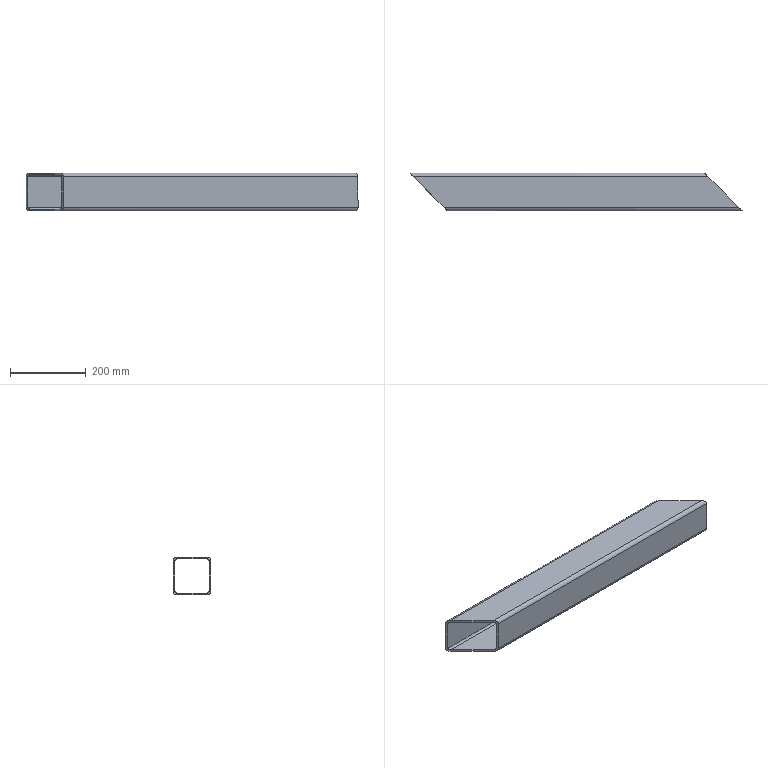Part | SolidWorks | features 3DProfileFeature 1, ICE 1, WeldMemberFeat 1, WeldmentFeature 1 | 1 solid | 18 faces | box 877.817 x 100 x 100 mm | volume 1427777 mm3 | plane 10 | cylinder 8 | commonest cylinder face diameters 10 x4 20 x4
STEP:
#1=CARTESIAN_POINT('',(777.817,50.,-40.));
#2=VERTEX_POINT('',#1);
#3=CARTESIAN_POINT('',(0.,50.,-40.));
#4=VERTEX_POINT('',#3);
#5=CARTESIAN_POINT('',(900.,50.,-40.));
#6=DIRECTION('',(-1.,0.,0.));
#7=VECTOR('',#6,1000.);
#8=LINE('',#5,#7);
#9=EDGE_CURVE('',#2,#4,#8,.T.);
#10=ORIENTED_EDGE('',*,*,#9,.F.);
#11=CARTESIAN_POINT('',(787.817,40.,-50.));
#12=VERTEX_POINT('',#11);
#13=CARTESIAN_POINT('',(777.817,50.,-40.));
#14=CARTESIAN_POINT('',(777.817,50.,-45.858));
#15=CARTESIAN_POINT('',(781.96,45.858,-50.));
#16=CARTESIAN_POINT('',(787.817,40.,-50.));
#17=(BOUNDED_CURVE()B_SPLINE_CURVE(3,(#13,#14,#15,#16),.UNSPECIFIED.,.F.,.T.)B_SPLINE_CURVE_WITH_KNOTS((4,4),(0.,1.571),.UNSPECIFIED.)CURVE()GEOMETRIC_REPRESENTATION_ITEM()RATIONAL_B_SPLINE_CURVE((1.,0.8047,0.8047,1.))REPRESENTATION_ITEM(''));
#18=EDGE_CURVE('',#2,#12,#17,.T.);
#19=ORIENTED_EDGE('',*,*,#18,.T.);
#20=CARTESIAN_POINT('',(10.,40.,-50.));
#21=VERTEX_POINT('',#20);
#22=CARTESIAN_POINT('',(900.,40.,-50.));
#23=DIRECTION('',(-1.,0.,0.));
#24=VECTOR('',#23,1000.);
#25=LINE('',#22,#24);
#26=EDGE_CURVE('',#12,#21,#25,.T.);
#27=ORIENTED_EDGE('',*,*,#26,.T.);
#28=CARTESIAN_POINT('',(10.,40.,-50.));
#29=CARTESIAN_POINT('',(4.142,45.858,-50.));
#30=CARTESIAN_POINT('',(0.,50.,-45.858));
#31=CARTESIAN_POINT('',(0.,50.,-40.));
#32=(BOUNDED_CURVE()B_SPLINE_CURVE(3,(#28,#29,#30,#31),.UNSPECIFIED.,.F.,.T.)B_SPLINE_CURVE_WITH_KNOTS((4,4),(4.712,6.283),.UNSPECIFIED.)CURVE()GEOMETRIC_REPRESENTATION_ITEM()RATIONAL_B_SPLINE_CURVE((1.,0.8047,0.8047,1.))REPRESENTATION_ITEM(''));
#33=EDGE_CURVE('',#21,#4,#32,.T.);
#34=ORIENTED_EDGE('',*,*,#33,.T.);
#35=EDGE_LOOP('',(#10,#19,#27,#34));
#36=FACE_OUTER_BOUND('',#35,.T.);
#37=CARTESIAN_POINT('',(900.,40.,-40.));
#38=DIRECTION('',(-1.,0.,0.));
#39=DIRECTION('',(0.,0.,1.));
#40=AXIS2_PLACEMENT_3D('',#37,#38,#39);
#41=CYLINDRICAL_SURFACE('',#40,10.);
#42=ADVANCED_FACE('',(#36),#41,.T.);
#43=CARTESIAN_POINT('',(777.817,50.,40.));
#44=VERTEX_POINT('',#43);
#45=CARTESIAN_POINT('',(0.,50.,40.));
#46=VERTEX_POINT('',#45);
#47=CARTESIAN_POINT('',(900.,50.,40.));
#48=DIRECTION('',(-1.,0.,0.));
#49=VECTOR('',#48,1000.);
#50=LINE('',#47,#49);
#51=EDGE_CURVE('',#44,#46,#50,.T.);
#52=ORIENTED_EDGE('',*,*,#51,.F.);
#53=CARTESIAN_POINT('',(777.817,50.,-50.));
#54=DIRECTION('',(0.,0.,1.));
#55=VECTOR('',#54,1000.);
#56=LINE('',#53,#55);
#57=EDGE_CURVE('',#2,#44,#56,.T.);
#58=ORIENTED_EDGE('',*,*,#57,.F.);
#59=ORIENTED_EDGE('',*,*,#9,.T.);
#60=CARTESIAN_POINT('',(0.,50.,-40.));
#61=DIRECTION('',(0.,0.,1.));
#62=VECTOR('',#61,1000.);
#63=LINE('',#60,#62);
#64=EDGE_CURVE('',#4,#46,#63,.T.);
#65=ORIENTED_EDGE('',*,*,#64,.T.);
#66=EDGE_LOOP('',(#52,#58,#59,#65));
#67=FACE_OUTER_BOUND('',#66,.T.);
#68=CARTESIAN_POINT('',(900.,50.,-40.));
#69=DIRECTION('',(0.,-1.,0.));
#70=DIRECTION('',(0.,0.,-1.));
#71=AXIS2_PLACEMENT_3D('',#68,#69,#70);
#72=PLANE('',#71);
#73=ADVANCED_FACE('',(#67),#72,.F.);
#74=CARTESIAN_POINT('',(787.817,40.,50.));
#75=VERTEX_POINT('',#74);
#76=CARTESIAN_POINT('',(10.,40.,50.));
#77=VERTEX_POINT('',#76);
#78=CARTESIAN_POINT('',(900.,40.,50.));
#79=DIRECTION('',(-1.,0.,0.));
#80=VECTOR('',#79,1000.);
#81=LINE('',#78,#80);
#82=EDGE_CURVE('',#75,#77,#81,.T.);
#83=ORIENTED_EDGE('',*,*,#82,.F.);
#84=CARTESIAN_POINT('',(787.817,40.,50.));
#85=CARTESIAN_POINT('',(781.96,45.858,50.));
#86=CARTESIAN_POINT('',(777.817,50.,45.858));
#87=CARTESIAN_POINT('',(777.817,50.,40.));
#88=(BOUNDED_CURVE()B_SPLINE_CURVE(3,(#84,#85,#86,#87),.UNSPECIFIED.,.F.,.T.)B_SPLINE_CURVE_WITH_KNOTS((4,4),(4.712,6.283),.UNSPECIFIED.)CURVE()GEOMETRIC_REPRESENTATION_ITEM()RATIONAL_B_SPLINE_CURVE((1.,0.8047,0.8047,1.))REPRESENTATION_ITEM(''));
#89=EDGE_CURVE('',#75,#44,#88,.T.);
#90=ORIENTED_EDGE('',*,*,#89,.T.);
#91=ORIENTED_EDGE('',*,*,#51,.T.);
#92=CARTESIAN_POINT('',(0.,50.,40.));
#93=CARTESIAN_POINT('',(0.,50.,45.858));
#94=CARTESIAN_POINT('',(4.142,45.858,50.));
#95=CARTESIAN_POINT('',(10.,40.,50.));
#96=(BOUNDED_CURVE()B_SPLINE_CURVE(3,(#92,#93,#94,#95),.UNSPECIFIED.,.F.,.T.)B_SPLINE_CURVE_WITH_KNOTS((4,4),(0.,1.571),.UNSPECIFIED.)CURVE()GEOMETRIC_REPRESENTATION_ITEM()RATIONAL_B_SPLINE_CURVE((1.,0.8047,0.8047,1.))REPRESENTATION_ITEM(''));
#97=EDGE_CURVE('',#46,#77,#96,.T.);
#98=ORIENTED_EDGE('',*,*,#97,.T.);
#99=EDGE_LOOP('',(#83,#90,#91,#98));
#100=FACE_OUTER_BOUND('',#99,.T.);
#101=CARTESIAN_POINT('',(900.,40.,40.));
#102=DIRECTION('',(-1.,0.,0.));
#103=DIRECTION('',(0.,0.,1.));
#104=AXIS2_PLACEMENT_3D('',#101,#102,#103);
#105=CYLINDRICAL_SURFACE('',#104,10.);
#106=ADVANCED_FACE('',(#100),#105,.T.);
#107=CARTESIAN_POINT('',(867.817,-40.,50.));
#108=VERTEX_POINT('',#107);
#109=CARTESIAN_POINT('',(90.,-40.,50.));
#110=VERTEX_POINT('',#109);
#111=CARTESIAN_POINT('',(900.,-40.,50.));
#112=DIRECTION('',(-1.,0.,0.));
#113=VECTOR('',#112,1000.);
#114=LINE('',#111,#113);
#115=EDGE_CURVE('',#108,#110,#114,.T.);
#116=ORIENTED_EDGE('',*,*,#115,.F.);
#117=CARTESIAN_POINT('',(777.817,50.,50.));
#118=DIRECTION('',(0.7071,-0.7071,0.));
#119=VECTOR('',#118,1000.);
#120=LINE('',#117,#119);
#121=EDGE_CURVE('',#75,#108,#120,.T.);
#122=ORIENTED_EDGE('',*,*,#121,.F.);
#123=ORIENTED_EDGE('',*,*,#82,.T.);
#124=CARTESIAN_POINT('',(0.,50.,50.));
#125=DIRECTION('',(-0.7071,0.7071,0.));
#126=VECTOR('',#125,1000.);
#127=LINE('',#124,#126);
#128=EDGE_CURVE('',#110,#77,#127,.T.);
#129=ORIENTED_EDGE('',*,*,#128,.F.);
#130=EDGE_LOOP('',(#116,#122,#123,#129));
#131=FACE_OUTER_BOUND('',#130,.T.);
#132=CARTESIAN_POINT('',(900.,-40.,50.));
#133=DIRECTION('',(0.,0.,-1.));
#134=DIRECTION('',(-1.,0.,0.));
#135=AXIS2_PLACEMENT_3D('',#132,#133,#134);
#136=PLANE('',#135);
#137=ADVANCED_FACE('',(#131),#136,.F.);
#138=CARTESIAN_POINT('',(877.817,-50.,40.));
#139=VERTEX_POINT('',#138);
#140=CARTESIAN_POINT('',(100.,-50.,40.));
#141=VERTEX_POINT('',#140);
#142=CARTESIAN_POINT('',(900.,-50.,40.));
#143=DIRECTION('',(-1.,0.,0.));
#144=VECTOR('',#143,1000.);
#145=LINE('',#142,#144);
#146=EDGE_CURVE('',#139,#141,#145,.T.);
#147=ORIENTED_EDGE('',*,*,#146,.F.);
#148=CARTESIAN_POINT('',(877.817,-50.,40.));
#149=CARTESIAN_POINT('',(877.817,-50.,45.858));
#150=CARTESIAN_POINT('',(873.675,-45.858,50.));
#151=CARTESIAN_POINT('',(867.817,-40.,50.));
#152=(BOUNDED_CURVE()B_SPLINE_CURVE(3,(#148,#149,#150,#151),.UNSPECIFIED.,.F.,.T.)B_SPLINE_CURVE_WITH_KNOTS((4,4),(3.142,4.712),.UNSPECIFIED.)CURVE()GEOMETRIC_REPRESENTATION_ITEM()RATIONAL_B_SPLINE_CURVE((1.,0.8047,0.8047,1.))REPRESENTATION_ITEM(''));
#153=EDGE_CURVE('',#139,#108,#152,.T.);
#154=ORIENTED_EDGE('',*,*,#153,.T.);
#155=ORIENTED_EDGE('',*,*,#115,.T.);
#156=CARTESIAN_POINT('',(90.,-40.,50.));
#157=CARTESIAN_POINT('',(95.858,-45.858,50.));
#158=CARTESIAN_POINT('',(100.,-50.,45.858));
#159=CARTESIAN_POINT('',(100.,-50.,40.));
#160=(BOUNDED_CURVE()B_SPLINE_CURVE(3,(#156,#157,#158,#159),.UNSPECIFIED.,.F.,.T.)B_SPLINE_CURVE_WITH_KNOTS((4,4),(1.571,3.142),.UNSPECIFIED.)CURVE()GEOMETRIC_REPRESENTATION_ITEM()RATIONAL_B_SPLINE_CURVE((1.,0.8047,0.8047,1.))REPRESENTATION_ITEM(''));
#161=EDGE_CURVE('',#110,#141,#160,.T.);
#162=ORIENTED_EDGE('',*,*,#161,.T.);
#163=EDGE_LOOP('',(#147,#154,#155,#162));
#164=FACE_OUTER_BOUND('',#163,.T.);
#165=CARTESIAN_POINT('',(900.,-40.,40.));
#166=DIRECTION('',(-1.,0.,0.));
#167=DIRECTION('',(0.,0.,1.));
#168=AXIS2_PLACEMENT_3D('',#165,#166,#167);
#169=CYLINDRICAL_SURFACE('',#168,10.);
#170=ADVANCED_FACE('',(#164),#169,.T.);
#171=CARTESIAN_POINT('',(877.817,-50.,-40.));
#172=VERTEX_POINT('',#171);
#173=CARTESIAN_POINT('',(100.,-50.,-40.));
#174=VERTEX_POINT('',#173);
#175=CARTESIAN_POINT('',(900.,-50.,-40.));
#176=DIRECTION('',(-1.,0.,0.));
#177=VECTOR('',#176,1000.);
#178=LINE('',#175,#177);
#179=EDGE_CURVE('',#172,#174,#178,.T.);
#180=ORIENTED_EDGE('',*,*,#179,.F.);
#181=CARTESIAN_POINT('',(877.817,-50.,40.));
#182=DIRECTION('',(0.,0.,1.));
#183=VECTOR('',#182,1000.);
#184=LINE('',#181,#183);
#185=EDGE_CURVE('',#172,#139,#184,.T.);
#186=ORIENTED_EDGE('',*,*,#185,.T.);
#187=ORIENTED_EDGE('',*,*,#146,.T.);
#188=CARTESIAN_POINT('',(100.,-50.,-50.));
#189=DIRECTION('',(0.,0.,1.));
#190=VECTOR('',#189,1000.);
#191=LINE('',#188,#190);
#192=EDGE_CURVE('',#174,#141,#191,.T.);
#193=ORIENTED_EDGE('',*,*,#192,.F.);
#194=EDGE_LOOP('',(#180,#186,#187,#193));
#195=FACE_OUTER_BOUND('',#194,.T.);
#196=CARTESIAN_POINT('',(900.,-50.,40.));
#197=DIRECTION('',(0.,1.,0.));
#198=DIRECTION('',(0.,0.,1.));
#199=AXIS2_PLACEMENT_3D('',#196,#197,#198);
#200=PLANE('',#199);
#201=ADVANCED_FACE('',(#195),#200,.F.);
#202=CARTESIAN_POINT('',(867.817,-40.,-50.));
#203=VERTEX_POINT('',#202);
#204=CARTESIAN_POINT('',(90.,-40.,-50.));
#205=VERTEX_POINT('',#204);
#206=CARTESIAN_POINT('',(900.,-40.,-50.));
#207=DIRECTION('',(-1.,0.,0.));
#208=VECTOR('',#207,1000.);
#209=LINE('',#206,#208);
#210=EDGE_CURVE('',#203,#205,#209,.T.);
#211=ORIENTED_EDGE('',*,*,#210,.F.);
#212=CARTESIAN_POINT('',(867.817,-40.,-50.));
#213=CARTESIAN_POINT('',(873.675,-45.858,-50.));
#214=CARTESIAN_POINT('',(877.817,-50.,-45.858));
#215=CARTESIAN_POINT('',(877.817,-50.,-40.));
#216=(BOUNDED_CURVE()B_SPLINE_CURVE(3,(#212,#213,#214,#215),.UNSPECIFIED.,.F.,.T.)B_SPLINE_CURVE_WITH_KNOTS((4,4),(1.571,3.142),.UNSPECIFIED.)CURVE()GEOMETRIC_REPRESENTATION_ITEM()RATIONAL_B_SPLINE_CURVE((1.,0.8047,0.8047,1.))REPRESENTATION_ITEM(''));
#217=EDGE_CURVE('',#203,#172,#216,.T.);
#218=ORIENTED_EDGE('',*,*,#217,.T.);
#219=ORIENTED_EDGE('',*,*,#179,.T.);
#220=CARTESIAN_POINT('',(100.,-50.,-40.));
#221=CARTESIAN_POINT('',(100.,-50.,-45.858));
#222=CARTESIAN_POINT('',(95.858,-45.858,-50.));
#223=CARTESIAN_POINT('',(90.,-40.,-50.));
#224=(BOUNDED_CURVE()B_SPLINE_CURVE(3,(#220,#221,#222,#223),.UNSPECIFIED.,.F.,.T.)B_SPLINE_CURVE_WITH_KNOTS((4,4),(3.142,4.712),.UNSPECIFIED.)CURVE()GEOMETRIC_REPRESENTATION_ITEM()RATIONAL_B_SPLINE_CURVE((1.,0.8047,0.8047,1.))REPRESENTATION_ITEM(''));
#225=EDGE_CURVE('',#174,#205,#224,.T.);
#226=ORIENTED_EDGE('',*,*,#225,.T.);
#227=EDGE_LOOP('',(#211,#218,#219,#226));
#228=FACE_OUTER_BOUND('',#227,.T.);
#229=CARTESIAN_POINT('',(900.,-40.,-40.));
#230=DIRECTION('',(-1.,0.,0.));
#231=DIRECTION('',(0.,0.,1.));
#232=AXIS2_PLACEMENT_3D('',#229,#230,#231);
#233=CYLINDRICAL_SURFACE('',#232,10.);
#234=ADVANCED_FACE('',(#228),#233,.T.);
#235=CARTESIAN_POINT('',(787.817,40.,45.));
#236=VERTEX_POINT('',#235);
#237=CARTESIAN_POINT('',(782.817,45.,40.));
#238=VERTEX_POINT('',#237);
#239=CARTESIAN_POINT('',(787.817,40.,45.));
#240=CARTESIAN_POINT('',(784.889,42.929,45.));
#241=CARTESIAN_POINT('',(782.817,45.,42.929));
#242=CARTESIAN_POINT('',(782.817,45.,40.));
#243=(BOUNDED_CURVE()B_SPLINE_CURVE(3,(#239,#240,#241,#242),.UNSPECIFIED.,.F.,.T.)B_SPLINE_CURVE_WITH_KNOTS((4,4),(4.712,6.283),.UNSPECIFIED.)CURVE()GEOMETRIC_REPRESENTATION_ITEM()RATIONAL_B_SPLINE_CURVE((1.,0.8047,0.8047,1.))REPRESENTATION_ITEM(''));
#244=EDGE_CURVE('',#236,#238,#243,.T.);
#245=ORIENTED_EDGE('',*,*,#244,.F.);
#246=CARTESIAN_POINT('',(10.,40.,45.));
#247=VERTEX_POINT('',#246);
#248=CARTESIAN_POINT('',(900.,40.,45.));
#249=DIRECTION('',(-1.,0.,0.));
#250=VECTOR('',#249,1000.);
#251=LINE('',#248,#250);
#252=EDGE_CURVE('',#236,#247,#251,.T.);
#253=ORIENTED_EDGE('',*,*,#252,.T.);
#254=CARTESIAN_POINT('',(5.,45.,40.));
#255=VERTEX_POINT('',#254);
#256=CARTESIAN_POINT('',(5.,45.,40.));
#257=CARTESIAN_POINT('',(5.,45.,42.929));
#258=CARTESIAN_POINT('',(7.071,42.929,45.));
#259=CARTESIAN_POINT('',(10.,40.,45.));
#260=(BOUNDED_CURVE()B_SPLINE_CURVE(3,(#256,#257,#258,#259),.UNSPECIFIED.,.F.,.T.)B_SPLINE_CURVE_WITH_KNOTS((4,4),(0.,1.571),.UNSPECIFIED.)CURVE()GEOMETRIC_REPRESENTATION_ITEM()RATIONAL_B_SPLINE_CURVE((1.,0.8047,0.8047,1.))REPRESENTATION_ITEM(''));
#261=EDGE_CURVE('',#255,#247,#260,.T.);
#262=ORIENTED_EDGE('',*,*,#261,.F.);
#263=CARTESIAN_POINT('',(900.,45.,40.));
#264=DIRECTION('',(-1.,0.,0.));
#265=VECTOR('',#264,1000.);
#266=LINE('',#263,#265);
#267=EDGE_CURVE('',#238,#255,#266,.T.);
#268=ORIENTED_EDGE('',*,*,#267,.F.);
#269=EDGE_LOOP('',(#245,#253,#262,#268));
#270=FACE_OUTER_BOUND('',#269,.T.);
#271=CARTESIAN_POINT('',(900.,40.,40.));
#272=DIRECTION('',(-1.,0.,0.));
#273=DIRECTION('',(0.,0.,1.));
#274=AXIS2_PLACEMENT_3D('',#271,#272,#273);
#275=CYLINDRICAL_SURFACE('',#274,5.);
#276=ADVANCED_FACE('',(#270),#275,.F.);
#277=CARTESIAN_POINT('',(782.817,45.,-40.));
#278=VERTEX_POINT('',#277);
#279=CARTESIAN_POINT('',(782.817,45.,-40.));
#280=DIRECTION('',(0.,0.,-1.));
#281=VECTOR('',#280,1000.);
#282=LINE('',#279,#281);
#283=EDGE_CURVE('',#238,#278,#282,.T.);
#284=ORIENTED_EDGE('',*,*,#283,.F.);
#285=ORIENTED_EDGE('',*,*,#267,.T.);
#286=CARTESIAN_POINT('',(5.,45.,-40.));
#287=VERTEX_POINT('',#286);
#288=CARTESIAN_POINT('',(5.,45.,-40.));
#289=DIRECTION('',(0.,0.,1.));
#290=VECTOR('',#289,1000.);
#291=LINE('',#288,#290);
#292=EDGE_CURVE('',#287,#255,#291,.T.);
#293=ORIENTED_EDGE('',*,*,#292,.F.);
#294=CARTESIAN_POINT('',(900.,45.,-40.));
#295=DIRECTION('',(-1.,0.,0.));
#296=VECTOR('',#295,1000.);
#297=LINE('',#294,#296);
#298=EDGE_CURVE('',#278,#287,#297,.T.);
#299=ORIENTED_EDGE('',*,*,#298,.F.);
#300=EDGE_LOOP('',(#284,#285,#293,#299));
#301=FACE_OUTER_BOUND('',#300,.T.);
#302=CARTESIAN_POINT('',(900.,45.,-40.));
#303=DIRECTION('',(0.,-1.,0.));
#304=DIRECTION('',(0.,0.,-1.));
#305=AXIS2_PLACEMENT_3D('',#302,#303,#304);
#306=PLANE('',#305);
#307=ADVANCED_FACE('',(#301),#306,.T.);
#308=CARTESIAN_POINT('',(787.817,40.,-45.));
#309=VERTEX_POINT('',#308);
#310=CARTESIAN_POINT('',(782.817,45.,-40.));
#311=CARTESIAN_POINT('',(782.817,45.,-42.929));
#312=CARTESIAN_POINT('',(784.889,42.929,-45.));
#313=CARTESIAN_POINT('',(787.817,40.,-45.));
#314=(BOUNDED_CURVE()B_SPLINE_CURVE(3,(#310,#311,#312,#313),.UNSPECIFIED.,.F.,.T.)B_SPLINE_CURVE_WITH_KNOTS((4,4),(0.,1.571),.UNSPECIFIED.)CURVE()GEOMETRIC_REPRESENTATION_ITEM()RATIONAL_B_SPLINE_CURVE((1.,0.8047,0.8047,1.))REPRESENTATION_ITEM(''));
#315=EDGE_CURVE('',#278,#309,#314,.T.);
#316=ORIENTED_EDGE('',*,*,#315,.F.);
#317=ORIENTED_EDGE('',*,*,#298,.T.);
#318=CARTESIAN_POINT('',(10.,40.,-45.));
#319=VERTEX_POINT('',#318);
#320=CARTESIAN_POINT('',(10.,40.,-45.));
#321=CARTESIAN_POINT('',(7.071,42.929,-45.));
#322=CARTESIAN_POINT('',(5.,45.,-42.929));
#323=CARTESIAN_POINT('',(5.,45.,-40.));
#324=(BOUNDED_CURVE()B_SPLINE_CURVE(3,(#320,#321,#322,#323),.UNSPECIFIED.,.F.,.T.)B_SPLINE_CURVE_WITH_KNOTS((4,4),(4.712,6.283),.UNSPECIFIED.)CURVE()GEOMETRIC_REPRESENTATION_ITEM()RATIONAL_B_SPLINE_CURVE((1.,0.8047,0.8047,1.))REPRESENTATION_ITEM(''));
#325=EDGE_CURVE('',#319,#287,#324,.T.);
#326=ORIENTED_EDGE('',*,*,#325,.F.);
#327=CARTESIAN_POINT('',(900.,40.,-45.));
#328=DIRECTION('',(-1.,0.,0.));
#329=VECTOR('',#328,1000.);
#330=LINE('',#327,#329);
#331=EDGE_CURVE('',#309,#319,#330,.T.);
#332=ORIENTED_EDGE('',*,*,#331,.F.);
#333=EDGE_LOOP('',(#316,#317,#326,#332));
#334=FACE_OUTER_BOUND('',#333,.T.);
#335=CARTESIAN_POINT('',(900.,40.,-40.));
#336=DIRECTION('',(-1.,0.,0.));
#337=DIRECTION('',(0.,0.,1.));
#338=AXIS2_PLACEMENT_3D('',#335,#336,#337);
#339=CYLINDRICAL_SURFACE('',#338,5.);
#340=ADVANCED_FACE('',(#334),#339,.F.);
#341=CARTESIAN_POINT('',(867.817,-40.,-45.));
#342=VERTEX_POINT('',#341);
#343=CARTESIAN_POINT('',(843.909,-16.091,-45.));
#344=DIRECTION('',(0.7071,-0.7071,0.));
#345=VECTOR('',#344,1000.);
#346=LINE('',#343,#345);
#347=EDGE_CURVE('',#309,#342,#346,.T.);
#348=ORIENTED_EDGE('',*,*,#347,.F.);
#349=ORIENTED_EDGE('',*,*,#331,.T.);
#350=CARTESIAN_POINT('',(90.,-40.,-45.));
#351=VERTEX_POINT('',#350);
#352=CARTESIAN_POINT('',(455.,-405.,-45.));
#353=DIRECTION('',(-0.7071,0.7071,0.));
#354=VECTOR('',#353,1000.);
#355=LINE('',#352,#354);
#356=EDGE_CURVE('',#351,#319,#355,.T.);
#357=ORIENTED_EDGE('',*,*,#356,.F.);
#358=CARTESIAN_POINT('',(900.,-40.,-45.));
#359=DIRECTION('',(-1.,0.,0.));
#360=VECTOR('',#359,1000.);
#361=LINE('',#358,#360);
#362=EDGE_CURVE('',#342,#351,#361,.T.);
#363=ORIENTED_EDGE('',*,*,#362,.F.);
#364=EDGE_LOOP('',(#348,#349,#357,#363));
#365=FACE_OUTER_BOUND('',#364,.T.);
#366=CARTESIAN_POINT('',(900.,40.,-45.));
#367=DIRECTION('',(0.,0.,1.));
#368=DIRECTION('',(1.,0.,0.));
#369=AXIS2_PLACEMENT_3D('',#366,#367,#368);
#370=PLANE('',#369);
#371=ADVANCED_FACE('',(#365),#370,.T.);
#372=CARTESIAN_POINT('',(872.817,-45.,-40.));
#373=VERTEX_POINT('',#372);
#374=CARTESIAN_POINT('',(867.817,-40.,-45.));
#375=CARTESIAN_POINT('',(870.746,-42.929,-45.));
#376=CARTESIAN_POINT('',(872.817,-45.,-42.929));
#377=CARTESIAN_POINT('',(872.817,-45.,-40.));
#378=(BOUNDED_CURVE()B_SPLINE_CURVE(3,(#374,#375,#376,#377),.UNSPECIFIED.,.F.,.F.)B_SPLINE_CURVE_WITH_KNOTS((4,4),(1.571,3.142),.UNSPECIFIED.)CURVE()GEOMETRIC_REPRESENTATION_ITEM()RATIONAL_B_SPLINE_CURVE((1.,0.8047,0.8047,1.))REPRESENTATION_ITEM(''));
#379=EDGE_CURVE('',#342,#373,#378,.T.);
#380=ORIENTED_EDGE('',*,*,#379,.F.);
#381=ORIENTED_EDGE('',*,*,#362,.T.);
#382=CARTESIAN_POINT('',(95.,-45.,-40.));
#383=VERTEX_POINT('',#382);
#384=CARTESIAN_POINT('',(95.,-45.,-40.));
#385=CARTESIAN_POINT('',(95.,-45.,-42.929));
#386=CARTESIAN_POINT('',(92.929,-42.929,-45.));
#387=CARTESIAN_POINT('',(90.,-40.,-45.));
#388=(BOUNDED_CURVE()B_SPLINE_CURVE(3,(#384,#385,#386,#387),.UNSPECIFIED.,.F.,.T.)B_SPLINE_CURVE_WITH_KNOTS((4,4),(3.142,4.712),.UNSPECIFIED.)CURVE()GEOMETRIC_REPRESENTATION_ITEM()RATIONAL_B_SPLINE_CURVE((1.,0.8047,0.8047,1.))REPRESENTATION_ITEM(''));
#389=EDGE_CURVE('',#383,#351,#388,.T.);
#390=ORIENTED_EDGE('',*,*,#389,.F.);
#391=CARTESIAN_POINT('',(900.,-45.,-40.));
#392=DIRECTION('',(-1.,0.,0.));
#393=VECTOR('',#392,1000.);
#394=LINE('',#391,#393);
#395=EDGE_CURVE('',#373,#383,#394,.T.);
#396=ORIENTED_EDGE('',*,*,#395,.F.);
#397=EDGE_LOOP('',(#380,#381,#390,#396));
#398=FACE_OUTER_BOUND('',#397,.T.);
#399=CARTESIAN_POINT('',(900.,-40.,-40.));
#400=DIRECTION('',(-1.,0.,0.));
#401=DIRECTION('',(0.,0.,1.));
#402=AXIS2_PLACEMENT_3D('',#399,#400,#401);
#403=CYLINDRICAL_SURFACE('',#402,5.);
#404=ADVANCED_FACE('',(#398),#403,.F.);
#405=CARTESIAN_POINT('',(872.817,-45.,40.));
#406=VERTEX_POINT('',#405);
#407=CARTESIAN_POINT('',(872.817,-45.,40.));
#408=DIRECTION('',(0.,0.,1.));
#409=VECTOR('',#408,1000.);
#410=LINE('',#407,#409);
#411=EDGE_CURVE('',#373,#406,#410,.T.);
#412=ORIENTED_EDGE('',*,*,#411,.F.);
#413=ORIENTED_EDGE('',*,*,#395,.T.);
#414=CARTESIAN_POINT('',(95.,-45.,40.));
#415=VERTEX_POINT('',#414);
#416=CARTESIAN_POINT('',(95.,-45.,40.));
#417=DIRECTION('',(0.,0.,-1.));
#418=VECTOR('',#417,1000.);
#419=LINE('',#416,#418);
#420=EDGE_CURVE('',#415,#383,#419,.T.);
#421=ORIENTED_EDGE('',*,*,#420,.F.);
#422=CARTESIAN_POINT('',(900.,-45.,40.));
#423=DIRECTION('',(-1.,0.,0.));
#424=VECTOR('',#423,1000.);
#425=LINE('',#422,#424);
#426=EDGE_CURVE('',#406,#415,#425,.T.);
#427=ORIENTED_EDGE('',*,*,#426,.F.);
#428=EDGE_LOOP('',(#412,#413,#421,#427));
#429=FACE_OUTER_BOUND('',#428,.T.);
#430=CARTESIAN_POINT('',(900.,-45.,40.));
#431=DIRECTION('',(0.,1.,0.));
#432=DIRECTION('',(0.,0.,1.));
#433=AXIS2_PLACEMENT_3D('',#430,#431,#432);
#434=PLANE('',#433);
#435=ADVANCED_FACE('',(#429),#434,.T.);
#436=CARTESIAN_POINT('',(867.817,-40.,45.));
#437=VERTEX_POINT('',#436);
#438=CARTESIAN_POINT('',(872.817,-45.,40.));
#439=CARTESIAN_POINT('',(872.817,-45.,42.929));
#440=CARTESIAN_POINT('',(870.746,-42.929,45.));
#441=CARTESIAN_POINT('',(867.817,-40.,45.));
#442=(BOUNDED_CURVE()B_SPLINE_CURVE(3,(#438,#439,#440,#441),.UNSPECIFIED.,.F.,.F.)B_SPLINE_CURVE_WITH_KNOTS((4,4),(3.142,4.712),.UNSPECIFIED.)CURVE()GEOMETRIC_REPRESENTATION_ITEM()RATIONAL_B_SPLINE_CURVE((1.,0.8047,0.8047,1.))REPRESENTATION_ITEM(''));
#443=EDGE_CURVE('',#406,#437,#442,.T.);
#444=ORIENTED_EDGE('',*,*,#443,.F.);
#445=ORIENTED_EDGE('',*,*,#426,.T.);
#446=CARTESIAN_POINT('',(90.,-40.,45.));
#447=VERTEX_POINT('',#446);
#448=CARTESIAN_POINT('',(90.,-40.,45.));
#449=CARTESIAN_POINT('',(92.929,-42.929,45.));
#450=CARTESIAN_POINT('',(95.,-45.,42.929));
#451=CARTESIAN_POINT('',(95.,-45.,40.));
#452=(BOUNDED_CURVE()B_SPLINE_CURVE(3,(#448,#449,#450,#451),.UNSPECIFIED.,.F.,.F.)B_SPLINE_CURVE_WITH_KNOTS((4,4),(1.571,3.142),.UNSPECIFIED.)CURVE()GEOMETRIC_REPRESENTATION_ITEM()RATIONAL_B_SPLINE_CURVE((1.,0.8047,0.8047,1.))REPRESENTATION_ITEM(''));
#453=EDGE_CURVE('',#447,#415,#452,.T.);
#454=ORIENTED_EDGE('',*,*,#453,.F.);
#455=CARTESIAN_POINT('',(900.,-40.,45.));
#456=DIRECTION('',(-1.,0.,0.));
#457=VECTOR('',#456,1000.);
#458=LINE('',#455,#457);
#459=EDGE_CURVE('',#437,#447,#458,.T.);
#460=ORIENTED_EDGE('',*,*,#459,.F.);
#461=EDGE_LOOP('',(#444,#445,#454,#460));
#462=FACE_OUTER_BOUND('',#461,.T.);
#463=CARTESIAN_POINT('',(900.,-40.,40.));
#464=DIRECTION('',(-1.,0.,0.));
#465=DIRECTION('',(0.,0.,1.));
#466=AXIS2_PLACEMENT_3D('',#463,#464,#465);
#467=CYLINDRICAL_SURFACE('',#466,5.);
#468=ADVANCED_FACE('',(#462),#467,.F.);
#469=CARTESIAN_POINT('',(883.909,-56.091,45.));
#470=DIRECTION('',(-0.7071,0.7071,0.));
#471=VECTOR('',#470,1000.);
#472=LINE('',#469,#471);
#473=EDGE_CURVE('',#437,#236,#472,.T.);
#474=ORIENTED_EDGE('',*,*,#473,.F.);
#475=ORIENTED_EDGE('',*,*,#459,.T.);
#476=CARTESIAN_POINT('',(495.,-445.,45.));
#477=DIRECTION('',(0.7071,-0.7071,0.));
#478=VECTOR('',#477,1000.);
#479=LINE('',#476,#478);
#480=EDGE_CURVE('',#247,#447,#479,.T.);
#481=ORIENTED_EDGE('',*,*,#480,.F.);
#482=ORIENTED_EDGE('',*,*,#252,.F.);
#483=EDGE_LOOP('',(#474,#475,#481,#482));
#484=FACE_OUTER_BOUND('',#483,.T.);
#485=CARTESIAN_POINT('',(900.,-40.,45.));
#486=DIRECTION('',(0.,0.,-1.));
#487=DIRECTION('',(-1.,0.,0.));
#488=AXIS2_PLACEMENT_3D('',#485,#486,#487);
#489=PLANE('',#488);
#490=ADVANCED_FACE('',(#484),#489,.T.);
#491=ORIENTED_EDGE('',*,*,#26,.F.);
#492=CARTESIAN_POINT('',(777.817,50.,-50.));
#493=DIRECTION('',(0.7071,-0.7071,0.));
#494=VECTOR('',#493,1000.);
#495=LINE('',#492,#494);
#496=EDGE_CURVE('',#12,#203,#495,.T.);
#497=ORIENTED_EDGE('',*,*,#496,.T.);
#498=ORIENTED_EDGE('',*,*,#210,.T.);
#499=CARTESIAN_POINT('',(0.,50.,-50.));
#500=DIRECTION('',(-0.7071,0.7071,0.));
#501=VECTOR('',#500,1000.);
#502=LINE('',#499,#501);
#503=EDGE_CURVE('',#205,#21,#502,.T.);
#504=ORIENTED_EDGE('',*,*,#503,.T.);
#505=EDGE_LOOP('',(#491,#497,#498,#504));
#506=FACE_OUTER_BOUND('',#505,.T.);
#507=CARTESIAN_POINT('',(900.,40.,-50.));
#508=DIRECTION('',(0.,0.,1.));
#509=DIRECTION('',(1.,0.,0.));
#510=AXIS2_PLACEMENT_3D('',#507,#508,#509);
#511=PLANE('',#510);
#512=ADVANCED_FACE('',(#506),#511,.F.);
#513=ORIENTED_EDGE('',*,*,#261,.T.);
#514=ORIENTED_EDGE('',*,*,#480,.T.);
#515=ORIENTED_EDGE('',*,*,#453,.T.);
#516=ORIENTED_EDGE('',*,*,#420,.T.);
#517=ORIENTED_EDGE('',*,*,#389,.T.);
#518=ORIENTED_EDGE('',*,*,#356,.T.);
#519=ORIENTED_EDGE('',*,*,#325,.T.);
#520=ORIENTED_EDGE('',*,*,#292,.T.);
#521=EDGE_LOOP('',(#513,#514,#515,#516,#517,#518,#519,#520));
#522=FACE_BOUND('',#521,.T.);
#523=ORIENTED_EDGE('',*,*,#503,.F.);
#524=ORIENTED_EDGE('',*,*,#225,.F.);
#525=ORIENTED_EDGE('',*,*,#192,.T.);
#526=ORIENTED_EDGE('',*,*,#161,.F.);
#527=ORIENTED_EDGE('',*,*,#128,.T.);
#528=ORIENTED_EDGE('',*,*,#97,.F.);
#529=ORIENTED_EDGE('',*,*,#64,.F.);
#530=ORIENTED_EDGE('',*,*,#33,.F.);
#531=EDGE_LOOP('',(#523,#524,#525,#526,#527,#528,#529,#530));
#532=FACE_OUTER_BOUND('',#531,.T.);
#533=CARTESIAN_POINT('',(0.,50.,-50.));
#534=DIRECTION('',(0.7071,0.7071,0.));
#535=DIRECTION('',(-0.7071,0.7071,0.));
#536=AXIS2_PLACEMENT_3D('',#533,#534,#535);
#537=PLANE('',#536);
#538=ADVANCED_FACE('',(#522,#532),#537,.F.);
#539=ORIENTED_EDGE('',*,*,#244,.T.);
#540=ORIENTED_EDGE('',*,*,#283,.T.);
#541=ORIENTED_EDGE('',*,*,#315,.T.);
#542=ORIENTED_EDGE('',*,*,#347,.T.);
#543=ORIENTED_EDGE('',*,*,#379,.T.);
#544=ORIENTED_EDGE('',*,*,#411,.T.);
#545=ORIENTED_EDGE('',*,*,#443,.T.);
#546=ORIENTED_EDGE('',*,*,#473,.T.);
#547=EDGE_LOOP('',(#539,#540,#541,#542,#543,#544,#545,#546));
#548=FACE_BOUND('',#547,.T.);
#549=ORIENTED_EDGE('',*,*,#57,.T.);
#550=ORIENTED_EDGE('',*,*,#89,.F.);
#551=ORIENTED_EDGE('',*,*,#121,.T.);
#552=ORIENTED_EDGE('',*,*,#153,.F.);
#553=ORIENTED_EDGE('',*,*,#185,.F.);
#554=ORIENTED_EDGE('',*,*,#217,.F.);
#555=ORIENTED_EDGE('',*,*,#496,.F.);
#556=ORIENTED_EDGE('',*,*,#18,.F.);
#557=EDGE_LOOP('',(#549,#550,#551,#552,#553,#554,#555,#556));
#558=FACE_OUTER_BOUND('',#557,.T.);
#559=CARTESIAN_POINT('',(777.817,50.,-50.));
#560=DIRECTION('',(-0.7071,-0.7071,0.));
#561=DIRECTION('',(0.7071,-0.7071,0.));
#562=AXIS2_PLACEMENT_3D('',#559,#560,#561);
#563=PLANE('',#562);
#564=ADVANCED_FACE('',(#548,#558),#563,.F.);
#565=CLOSED_SHELL('',(#42,#73,#106,#137,#170,#201,#234,#276,#307,#340,#371,#404,#435,#468,#490,#512,#538,#564));
#566=MANIFOLD_SOLID_BREP('',#565);
#567=CARTESIAN_POINT('',(0.,0.,0.));
#568=DIRECTION('',(0.,0.,1.));
#569=DIRECTION('',(1.,0.,0.));
#570=AXIS2_PLACEMENT_3D('',#567,#568,#569);
#571=(LENGTH_UNIT()NAMED_UNIT(*)SI_UNIT(.MILLI.,.METRE.));
#572=UNCERTAINTY_MEASURE_WITH_UNIT(LENGTH_MEASURE(0.00001),#571,'','');
#573=(NAMED_UNIT(*)PLANE_ANGLE_UNIT()SI_UNIT($,.RADIAN.));
#574=(NAMED_UNIT(*)SI_UNIT($,.STERADIAN.)SOLID_ANGLE_UNIT());
#575=(GEOMETRIC_REPRESENTATION_CONTEXT(3)GLOBAL_UNCERTAINTY_ASSIGNED_CONTEXT((#572))GLOBAL_UNIT_ASSIGNED_CONTEXT((#571,#573,#574))REPRESENTATION_CONTEXT('',''));
#576=ADVANCED_BREP_SHAPE_REPRESENTATION('',(#566,#570),#575);